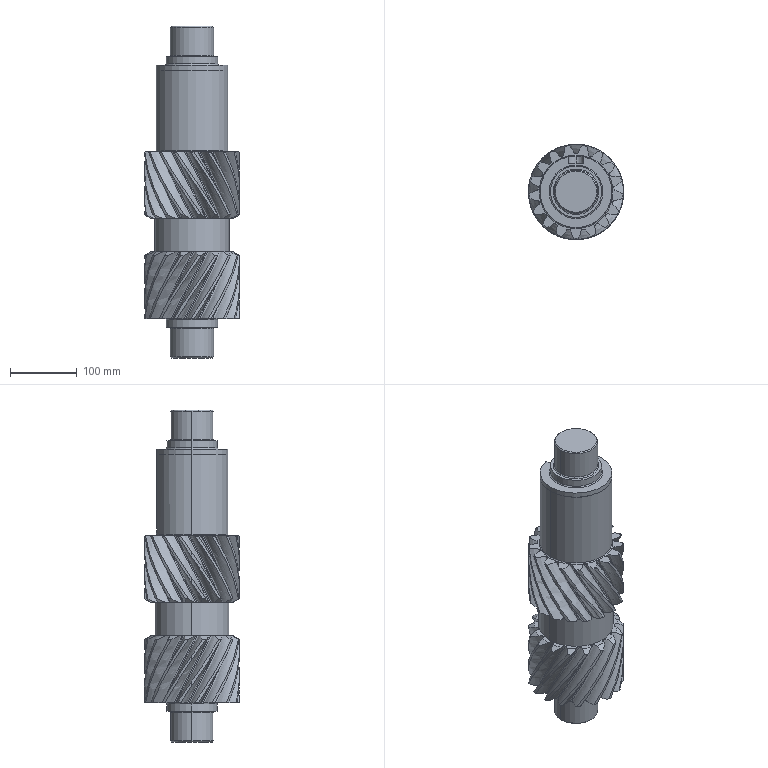Part | SolidWorks | features Chamfer 3, Fillet 2, ICE 2, CirPattern 1, Extrusion 1, Helix 1, MirrorSolid 1, RefAxis 1, Revolution 1, SweepCut 1 | 1 solid | 255 faces | box 142.951 x 142.951 x 498.475 mm | volume 4697605 mm3 | spline 102 | cone 74 | cylinder 56 | plane 13 | torus 10 | commonest cylinder face diameters 142.951 x38 65.011 x4 76.987 x4 107.696 x3 107.925 x3 22.225 x2